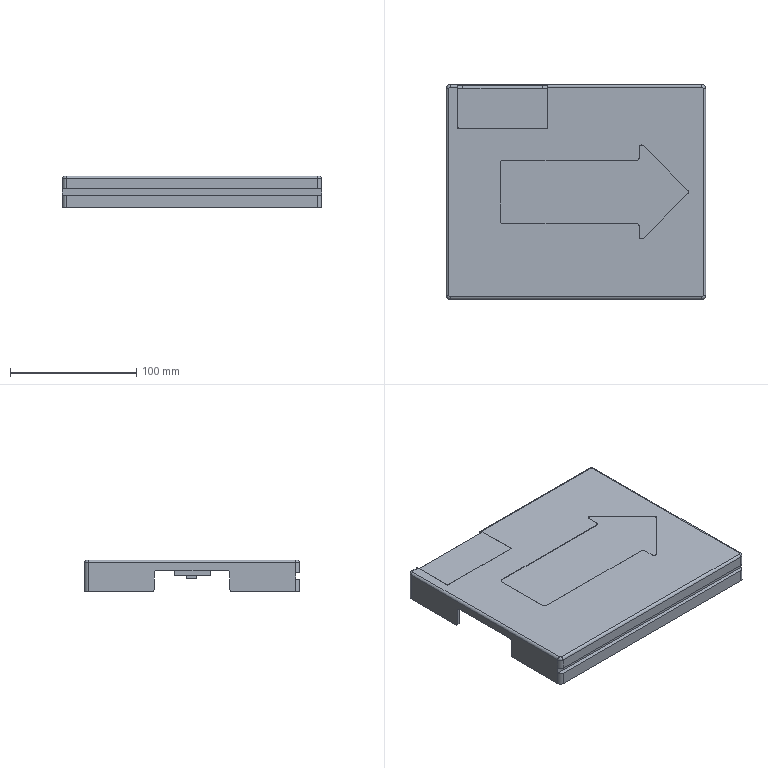NC program | NX | posted with a generic post | part box 205 x 170 x 25 mm
Lines 1976 to 3445 of 3445:
(CAVITY_MILL , TOOL : D4)
N3932 T17 M6
N3934 G54
N3936 G17 G0 G90 X-57.2 Y-18.808 B0. C0. S9500 M3
N3938 G43 Z30. H17
N3940 Z-0.25
N3942 G94 G1 X-57.5 Y-18.981 F1600.
N3944 G3 X-58. Y-19.847 R1.
N3946 G1 Y-23.
N3948 X-54.847
N3950 G3 X-53.981 Y-22.5 R1.
N3952 G1 X-53.808 Y-22.2
N3954 G0 X-57.2 Y-18.808 Z-0.5
N3956 G1 X-57.5 Y-18.981
N3958 G3 X-58. Y-19.847 R1.
N3960 G1 Y-23.
N3962 X-54.847
N3964 G3 X-53.981 Y-22.5 R1.
N3966 G1 X-53.808 Y-22.2
N3968 G0 Z30.
N3970 Y22.2
N3972 Z-0.25
N3974 G1 X-53.981 Y22.5
N3976 G3 X-54.847 Y23. R1.
N3978 G1 X-58.
N3980 Y19.847
N3982 G3 X-57.5 Y18.981 R1.
N3984 G1 X-57.2 Y18.808
N3986 G0 X-53.808 Y22.2 Z-0.5
N3988 G1 X-53.981 Y22.5
N3990 G3 X-54.847 Y23. R1.
N3992 G1 X-58.
N3994 Y19.847
N3996 G3 X-57.5 Y18.981 R1.
N3998 G1 X-57.2 Y18.808
N4000 G0 Z30.
N4002 X-87.339 Y53.756
N4004 Z-0.25
N4006 G1 X-88.048 Y52.529
N4008 G2 X-88.914 Y52.029 R1.
N4010 G1 X-89.48
N4012 Y52.678
N4014 G2 X-91.003 Y54.71 R2.52
N4016 G3 X-91.5 Y55.153 R0.5
N4018 G1 Y52.
N4020 X-88.347
N4022 X-88.348 Y52.029
N4024 X-88.914
N4026 G2 X-89.78 Y52.529 R1.
N4028 G1 X-90.162 Y54.558
N4030 G0 X-87.339 Y53.756 Z-0.5
N4032 G1 X-88.048 Y52.529
N4034 G2 X-88.914 Y52.029 R1.
N4036 G1 X-89.48
N4038 Y52.678
N4040 G2 X-91.003 Y54.71 R2.52
N4042 G3 X-91.5 Y55.153 R0.5
N4044 G1 Y52.
N4046 X-88.347
N4048 X-88.348 Y52.029
N4050 X-88.914
N4052 G2 X-89.78 Y52.529 R1.
N4054 G1 X-90.162 Y54.558
N4056 G0 X-87.339 Y53.756 Z-0.75
N4058 G1 X-88.048 Y52.529
N4060 G2 X-88.914 Y52.029 R1.
N4062 G1 X-89.48
N4064 Y52.678
N4066 G2 X-91.003 Y54.71 R2.52
N4068 G3 X-91.5 Y55.153 R0.5
N4070 G1 Y52.
N4072 X-88.347
N4074 X-88.348 Y52.029
N4076 X-88.914
N4078 G2 X-89.78 Y52.529 R1.
N4080 G1 X-90.162 Y54.558
N4082 G0 X-87.339 Y53.756 Z-1.
N4084 G1 X-88.048 Y52.529
N4086 G2 X-88.914 Y52.029 R1.
N4088 G1 X-89.48
N4090 Y52.678
N4092 G2 X-91.003 Y54.71 R2.52
N4094 G3 X-91.5 Y55.153 R0.5
N4096 G1 Y52.
N4098 X-88.347
N4100 X-88.348 Y52.029
N4102 X-88.914
N4104 G2 X-89.78 Y52.529 R1.
N4106 G1 X-90.162 Y54.558
N4108 G0 Z30.
N4110 X-25.837 Y54.56
N4112 Z-0.25
N4114 G1 X-26.22 Y52.529
N4116 G2 X-27.086 Y52.029 R1.
N4118 G1 X-27.652
N4120 X-27.653 Y52.
N4122 X-24.5
N4124 Y55.153
N4126 G3 X-24.997 Y54.71 R0.5
N4128 G2 X-26.518 Y52.679 R2.52
N4130 G1 X-26.519 Y52.029
N4132 X-27.086
N4134 G2 X-27.952 Y52.529 R1.
N4136 G1 X-28.66 Y53.756
N4138 G0 X-25.837 Y54.56 Z-0.5
N4140 G1 X-26.22 Y52.529
N4142 G2 X-27.086 Y52.029 R1.
N4144 G1 X-27.652
N4146 X-27.653 Y52.
N4148 X-24.5
N4150 Y55.153
N4152 G3 X-24.997 Y54.71 R0.5
N4154 G2 X-26.518 Y52.679 R2.52
N4156 G1 X-26.519 Y52.029
N4158 X-27.086
N4160 G2 X-27.952 Y52.529 R1.
N4162 G1 X-28.66 Y53.756
N4164 G0 X-25.837 Y54.56 Z-0.75
N4166 G1 X-26.22 Y52.529
N4168 G2 X-27.086 Y52.029 R1.
N4170 G1 X-27.652
N4172 X-27.653 Y52.
N4174 X-24.5
N4176 Y55.153
N4178 G3 X-24.997 Y54.71 R0.5
N4180 G2 X-26.518 Y52.679 R2.52
N4182 G1 X-26.519 Y52.029
N4184 X-27.086
N4186 G2 X-27.952 Y52.529 R1.
N4188 G1 X-28.66 Y53.756
N4190 G0 X-25.837 Y54.56 Z-1.
N4192 G1 X-26.22 Y52.529
N4194 G2 X-27.086 Y52.029 R1.
N4196 G1 X-27.652
N4198 X-27.653 Y52.
N4200 X-24.5
N4202 Y55.153
N4204 G3 X-24.997 Y54.71 R0.5
N4206 G2 X-26.518 Y52.679 R2.52
N4208 G1 X-26.519 Y52.029
N4210 X-27.086
N4212 G2 X-27.952 Y52.529 R1.
N4214 G1 X-28.66 Y53.756
N4216 G0 Z30.
N4218 X52.875 Y27.315
N4220 Z-0.25
N4222 G2 X52.497 Y28.218 R1.
N4224 X56.565 Y29.904 R2.52
N4226 G3 X57.23 Y29.942 R0.5
N4228 G1 X52. Y35.172
N4230 Y27.776
N4232 G3 X52.497 Y28.218 R0.5
N4234 G2 X53.093 Y29.021 R1.
N4236 G1 X53.508 Y28.784
N4238 G0 X52.875 Y27.315 Z-0.5
N4240 G2 X52.497 Y28.218 R1.
N4242 X56.565 Y29.904 R2.52
N4244 G3 X57.23 Y29.942 R0.5
N4246 G1 X52. Y35.172
N4248 Y27.776
N4250 G3 X52.497 Y28.218 R0.5
N4252 G2 X53.093 Y29.021 R1.
N4254 G1 X53.508 Y28.784
N4256 G0 Z30.
N4258 X83.642 Y-2.399
N4260 Z-0.25
N4262 G1 X83.976 Y-2.488
N4264 G3 X84.942 Y-2.23 R1.
N4266 G1 X87.172 Y0.
N4268 X84.942 Y2.23
N4270 G3 X83.976 Y2.488 R1.
N4272 G1 X83.642 Y2.399
N4274 G0 Y-2.399 Z-0.5
N4276 G1 X83.976 Y-2.488
N4278 G3 X84.942 Y-2.23 R1.
N4280 G1 X87.172 Y0.
N4282 X84.942 Y2.23
N4284 G3 X83.976 Y2.488 R1.
N4286 G1 X83.642 Y2.399
N4288 G0 Z30.
N4290 X55.021 Y-29.649
N4292 Z-0.25
N4294 G1 X55.027 Y-30.127
N4296 G2 X54.036 Y-30.257 R1.
N4298 X52.497 Y-28.218 R2.52
N4300 G3 X52. Y-27.776 R0.5
N4302 G1 Y-35.172
N4304 X57.23 Y-29.942
N4306 G3 X56.565 Y-29.904 R0.5
N4308 G2 X54.036 Y-30.257 R2.52
N4310 X53.427 Y-29.464 R1.
N4312 G1 X53.769 Y-29.13
N4314 G0 X55.021 Y-29.649 Z-0.5
N4316 G1 X55.027 Y-30.127
N4318 G2 X54.036 Y-30.257 R1.
N4320 X52.497 Y-28.218 R2.52
N4322 G3 X52. Y-27.776 R0.5
N4324 G1 Y-35.135
N4326 X52.002 Y-35.17
N4328 X57.23 Y-29.942
N4330 G3 X56.565 Y-29.904 R0.5
N4332 G2 X54.036 Y-30.257 R2.52
N4334 X53.427 Y-29.464 R1.
N4336 G1 X53.769 Y-29.13
N4338 G0 Z30.
N4340 M5
(FLOOR_WALL_1_COPY_1 , TOOL : D10JING)
N4342 T14 M6
N4344 G54
N4346 G17 G0 G90 X6.616 Y1. B0. C0. S9500 M3
N4348 G43 Z30. H14
N4350 Z1.
N4352 G94 G1 Z-0.5 F1000.
N4354 G3 X5.75 Y1.5 R1.
N4356 G1 X-36.5 F1200.
N4358 Y-1.5
N4360 X48.
N4362 G2 X54.44 Y-2.326 R25.5
N4364 G1 X56.766 Y0.
N4366 X54.44 Y2.326
N4368 G2 X48. Y1.5 R25.5
N4370 G1 X5.75
N4372 Y7.5
N4374 X-42.5
N4376 Y-7.5
N4378 X48.
N4380 G2 X56.024 Y-9.227 R19.5
N4382 G1 X65.251 Y0.
N4384 X56.024 Y9.227
N4386 G2 X48. Y7.5 R19.5
N4388 G1 X5.75
N4390 Y13.5
N4392 X-48.5
N4394 Y-13.5
N4396 X48.
N4398 G2 X56.893 Y-16.843 R13.5
N4400 G1 X73.737 Y0.
N4402 X56.893 Y16.843
N4404 G2 X48. Y13.5 R13.5
N4406 G1 X5.75
N4408 Y19.5
N4410 X-54.5
N4412 Y-19.5
N4414 X48.
N4416 G2 X55.495 Y-26.727 R7.5
N4418 G1 X82.222 Y0.
N4420 X55.495 Y26.727
N4422 G2 X48. Y19.5 R7.5
N4424 G1 X5.75
N4426 X6.616
N4428 G3 X5.75 Y20. R1. F1000.
N4430 G1 X-55. F1200.
N4432 Y-20.
N4434 X48.
N4436 G2 X55. Y-27. R7.
N4438 G1 Y-27.929
N4440 X82.929 Y0.
N4442 X55. Y27.929
N4444 Y27.
N4446 G2 X48. Y20. R7.
N4448 G1 X5.75
N4450 G3 X4.884 Y19.5 R1.
N4452 G1 X4.307 Y18.5
N4454 Z1.
N4456 G0 Z30.
N4458 X-52.029 Y70.
N4460 Z0.6
N4462 G1 X-58. Z-1. F1000.
N4464 X-76. F1200.
N4466 Y67.5
N4468 X-40.
N4470 Y70.
N4472 X-58.
N4474 Y76.
N4476 X-82.
N4478 Y61.5
N4480 X-34.
N4482 Y76.
N4484 X-58.
N4486 Y82.
N4488 X-88.
N4490 Y55.5
N4492 X-28.
N4494 Y82.
N4496 X-58.
N4498 G2 X-58.866 Y82.5 R1.
N4500 G1 X-62.33 Y88.5
N4502 Z0.5
N4504 X-86.5 Y80.5 F8000.
N4506 Z-1. F1000.
N4508 X-88. Y82.866
N4510 G3 X-88.5 Y82. R1.
N4512 G1 Y55. F1200.
N4514 X-27.5
N4516 Y82.
N4518 G3 X-28. Y82.866 R1.
N4520 G1 X-29.5 Y80.5
N4522 Z0.5
N4524 G0 Z30.
(ZLEVEL_PROFILE , TOOL : D10JING)
N4526 X101.868 Y-91.716
N4528 Z-9.5
N4530 G1 Z-12.5 F1000.
N4532 X100.984 Y-90.414
N4534 G3 X100.084 Y-89.979 R1.
N4536 G2 X99.497 Y-90. R8.
N4538 G1 X-99.498
N4540 G2 X-99.784 Y-89.995 R5.003
N4542 X-107.5 Y-81.986 R8.
N4544 G1 Y81.86
N4546 X-107.498
N4548 X-107.5 Y82.
N4550 G2 X-99.498 Y90. R8.
N4552 G1 X99.498
N4554 G2 X107.5 Y82. R8.
N4556 G1 X107.498 Y81.86
N4558 X107.5
N4560 Y-82.
N4562 G2 X100.084 Y-89.979 R8.
N4564 G3 X99.256 Y-90.541 R1.
N4566 G1 X98.55 Y-92.
N4568 Z-9.5
N4570 G0 X101.868 Y-91.716 Z-22.
N4572 G1 Z-25.
N4574 X100.984 Y-90.414
N4576 G3 X100.084 Y-89.979 R1.
N4578 G2 X99.497 Y-90. R8.
N4580 G1 X-99.498
N4582 G2 X-99.784 Y-89.995 R5.003
N4584 X-107.5 Y-81.986 R8.
N4586 G1 Y81.86
N4588 X-107.498
N4590 X-107.5 Y82.
N4592 G2 X-99.498 Y90. R8.
N4594 G1 X99.498
N4596 G2 X107.5 Y82. R8.
N4598 G1 X107.498 Y81.86
N4600 X107.5
N4602 Y-82.
N4604 G2 X100.084 Y-89.979 R8.
N4606 G3 X99.256 Y-90.541 R1.
N4608 G1 X98.55 Y-92.
N4610 Z-22.
N4612 G0 Z30.
N4614 M5
(ZLEVEL_PROFILE_1 , TOOL : D3R0.5)
N4616 T07 M6
N4618 G54
N4620 G17 G0 G90 X-23.737 Y84.233 B0. C0. S9500 M3
N4622 G43 Z30. H7
N4624 Z0.995
N4626 G94 G1 Z-0.005 F1000.
N4628 X-23.304 Y83.999
N4630 G3 X-23.004 Y84.006 R0.3
N4632 G2 X-22.5 Y84.147 R0.952 F2500.
N4634 G1 X99.499
N4636 G2 X101.647 Y82. R2.147
N4638 G1 X101.59 Y-81.871
N4640 X101.647 Y-82.
N4642 G2 X99.499 Y-84.147 R2.147
N4644 G1 X-99.499
N4646 G2 X-101.647 Y-82. R2.147
N4648 G1 X-101.59 Y81.137
N4650 Y81.871
N4652 X-101.647 Y82.
N4654 G2 X-99.499 Y84.147 R2.147
N4656 G1 X-93.5
N4658 G2 X-92.636 Y83.716 R1.144
N4660 G1 X-92.602 Y83.673
N4662 X-92.55 Y83.652
N4664 X-92.496 Y83.661
N4666 X-91.835 Y83.76
N4668 Z0.995
N4670 G0 Z30.
N4672 X-92.331 Y84.413
N4674 Z0.99
N4676 G1 Z-0.01 F1000.
N4678 X-92.701 Y84.13
N4680 G2 X-92.999 Y84.092 R0.3
N4682 G1 X-93.083 Y84.127 F2500.
N4684 X-93.5 Y84.223
N4686 X-99.499
N4688 G3 X-101.723 Y82. R2.223
N4690 G1 X-101.662 Y81.871
N4692 Y81.137
N4694 X-101.723 Y-82.
N4696 G3 X-99.5 Y-84.223 R2.223
N4698 G1 X99.5
N4700 G3 X101.723 Y-82. R2.223
N4702 G1 X101.662 Y-81.871
N4704 X101.723 Y82.
N4706 G3 X99.499 Y84.223 R2.223
N4708 G1 X-22.5
N4710 X-23. Y84.089
N4712 X-23.001 Y84.13 Z-0.013
N4714 Y84.142 Z-0.017
N4716 G2 X-22.5 Y84.287 R0.946
N4718 G1 X99.501
N4720 G2 X101.787 Y82. R2.287
N4722 G1 Y-82.
N4724 G2 X99.501 Y-84.287 R2.287
N4726 G1 X-99.501
N4728 G2 X-101.787 Y-82. R2.287
N4730 G1 Y82.
N4732 G2 X-99.499 Y84.287 R2.287
N4734 G1 X-93.5
N4736 X-93.073 Y84.197
N4738 X-92.996 Y84.143
N4740 X-92.987 Y84.197 Z-0.024
N4742 X-93.066 Y84.248
N4744 X-93.5 Y84.346
N4746 X-99.499
N4748 G3 X-101.846 Y82. R2.346
N4750 G1 Y-82.
N4752 G3 X-99.499 Y-84.346 R2.346
N4754 G1 X99.499
N4756 G3 X101.846 Y-82. R2.346
N4758 G1 Y82.
N4760 G3 X99.499 Y84.346 R2.346
N4762 G1 X-22.5
N4764 G3 X-23.001 Y84.202 R0.892
N4766 G1 Y84.277 Z-0.033
N4768 X-22.925 Y84.318
N4770 X-22.5 Y84.407
N4772 X99.499
N4774 G2 X101.907 Y82. R2.407
N4776 G1 Y-82.
N4778 G2 X99.499 Y-84.407 R2.407
N4780 G1 X-99.499
N4782 G2 X-101.907 Y-82. R2.407
N4784 G1 Y82.
N4786 G2 X-99.499 Y84.407 R2.407
N4788 G1 X-93.5
N4790 X-93.058 Y84.312
N4792 X-92.975 Y84.264
N4794 X-93. Y84.348 Z-0.045
N4796 G3 X-93.5 Y84.474 R2.086
N4798 G1 X-99.499
N4800 G3 X-101.974 Y82. R2.474
N4802 G1 Y-82.
N4804 G3 X-99.5 Y-84.474 R2.474
N4806 G1 X99.5
N4808 G3 X101.974 Y-82. R2.474
N4810 G1 Y82.
N4812 G3 X99.499 Y84.474 R2.474
N4814 G1 X-22.5
N4816 G3 X-23.001 Y84.35 R1.112
N4818 G1 Y84.421 Z-0.061
N4820 G2 X-22.5 Y84.549 R1.049
N4822 G1 X99.499
N4824 G2 X102.049 Y82. R2.549
N4826 G1 Y-82.
N4828 G2 X99.501 Y-84.549 R2.549
N4830 G1 X-99.501
N4832 G2 X-102.049 Y-82. R2.549
N4834 G1 Y82.
N4836 G2 X-99.501 Y84.549 R2.549
N4838 G1 X-93.5
N4840 G2 X-93. Y84.419 R2.188
N4842 G1 Y84.507 Z-0.081
N4844 G3 X-93.5 Y84.63 R1.14
N4846 G1 X-99.5
N4848 G3 X-102.13 Y82. R2.63
N4850 G1 Y-82.
N4852 G3 X-99.499 Y-84.63 R2.63
N4854 G1 X99.499
N4856 G3 X102.13 Y-82. R2.63
N4858 G1 Y82.
N4860 G3 X99.5 Y84.63 R2.63
N4862 G1 X-22.5
N4864 G3 X-23.001 Y84.509 R1.123
N4866 G1 X-22.963 Y84.572 Z-0.092
N4868 X-22.916 Y84.61 Z-0.104
N4870 X-22.5 Y84.697
N4872 X99.5
N4874 G2 X102.197 Y82. R2.697
N4876 G1 Y-82.
N4878 G2 X99.5 Y-84.697 R2.697
N4880 G1 X-99.5
N4882 G2 X-102.197 Y-82. R2.697
N4884 G1 Y82.
N4886 G2 X-99.5 Y84.697 R2.697
N4888 G1 X-93.5
N4890 X-93. Y84.579
N4892 Y84.639 Z-0.117
N4894 Y84.673 Z-0.13
N4896 X-93.5 Y84.795
N4898 X-99.5
N4900 G3 X-102.295 Y82. R2.795
N4902 G1 Y-82.
N4904 G3 X-99.501 Y-84.795 R2.795
N4906 G1 X99.501
N4908 G3 X102.295 Y-82. R2.795
N4910 G1 Y82.
N4912 G3 X99.5 Y84.795 R2.795
N4914 G1 X-22.5
N4916 X-22.921 Y84.704
N4918 X-22.948 Y84.782 Z-0.158
N4920 X-22.868 Y84.816
N4922 X-22.5 Y84.875
N4924 X99.5
N4926 G2 X102.375 Y82. R2.875
N4928 G1 Y-82.
N4930 G2 X99.499 Y-84.875 R2.875
N4932 G1 X-99.499
N4934 G2 X-102.375 Y-82. R2.875
N4936 G1 Y82.
N4938 G2 X-99.5 Y84.875 R2.875
N4940 G1 X-93.5
N4942 X-93.058 Y84.786
N4944 X-93. Y84.76
N4946 X-92.999 Y84.853 Z-0.192
N4948 X-93.5 Y84.96
N4950 X-99.5
N4952 G3 X-102.46 Y82. R2.96
N4954 G1 Y-82.
N4956 G3 X-99.5 Y-84.96 R2.96
N4958 G1 X99.5
N4960 G3 X102.46 Y-82. R2.96
N4962 G1 Y82.
N4964 G3 X99.5 Y84.96 R2.96
N4966 G1 X-22.5
N4968 G3 X-23. Y84.846 R8.99
N4970 G1 Y84.898 Z-0.21
N4972 X-23.001 Y84.931 Z-0.229
N4974 G2 X-22.5 Y85.045 R1.121
N4976 G1 X99.5
N4978 G2 X102.545 Y82. R3.045
N4980 G1 Y-82.
N4982 G2 X99.501 Y-85.045 R3.045
N4984 G1 X-99.501
N4986 G2 X-102.545 Y-82. R3.045
N4988 G1 Y82.
N4990 G2 X-99.5 Y85.045 R3.045
N4992 G1 X-93.5
N4994 X-92.999 Y84.943
N4996 Y84.984 Z-0.249
N4998 X-93. Y85.025 Z-0.269
N5000 X-93.084 Y85.053
N5002 X-93.5 Y85.129
N5004 X-99.5
N5006 G3 X-102.629 Y82. R3.129
N5008 G1 Y-82.
N5010 G3 X-99.5 Y-85.129 R3.129
N5012 G1 X99.5
N5014 G3 X102.629 Y-82. R3.129
N5016 G1 Y82.
N5018 G3 X99.5 Y85.129 R3.129
N5020 G1 X-22.5
N5022 X-22.923 Y85.053
N5024 X-23.001 Y85.022
N5026 X-22.943 Y85.083 Z-0.291
N5028 X-22.885 Y85.142 Z-0.313
N5030 X-22.5 Y85.212
N5032 X99.5
N5034 G2 X102.712 Y82. R3.212
N5036 G1 Y-82.
N5038 G2 X99.5 Y-85.212 R3.212
N5040 G1 X-99.5
N5042 G2 X-102.712 Y-82. R3.212
N5044 G1 Y82.
N5046 G2 X-99.5 Y85.212 R3.212
N5048 G1 X-93.5
N5050 G2 X-93. Y85.109 R5.057
N5052 G1 Y85.152 Z-0.337
N5054 Y85.197 Z-0.361
N5056 G3 X-93.5 Y85.294 R5.188
N5058 G1 X-99.5
N5060 G3 X-102.794 Y82. R3.294
N5062 G1 Y-82.
N5064 G3 X-99.501 Y-85.294 R3.294
N5066 G1 X99.501
N5068 G3 X102.794 Y-82. R3.294
N5070 G1 Y82.
N5072 G3 X99.5 Y85.294 R3.294
N5074 G1 X-22.5
N5076 X-22.885 Y85.23
N5078 X-22.939 Y85.256 Z-0.387
N5080 X-22.995 Y85.295 Z-0.412
N5082 X-22.5 Y85.375
N5084 X99.5
N5086 G2 X102.875 Y82. R3.375
N5088 G1 Y-82.
N5090 G2 X99.5 Y-85.375 R3.375
N5092 G1 X-99.5
N5094 G2 X-102.875 Y-82. R3.375
N5096 G1 Y82.
N5098 G2 X-99.5 Y85.375 R3.375
N5100 G1 X-93.5
N5102 X-93. Y85.292
N5104 Y85.342 Z-0.44
N5106 X-92.999 Y85.376 Z-0.467
N5108 X-93.5 Y85.455
N5110 X-99.5
N5112 G3 X-102.955 Y82. R3.455
N5114 G1 Y-82.
N5116 G3 X-99.5 Y-85.455 R3.455
N5118 G1 X99.5
N5120 G3 X102.955 Y-82. R3.455
N5122 G1 Y82.
N5124 G3 X99.5 Y85.455 R3.455
N5126 G1 X-22.5
N5128 X-23.002 Y85.378
N5130 Y85.419 Z-0.496
N5132 Y85.457 Z-0.525
N5134 X-22.5 Y85.533
N5136 X99.5
N5138 G2 X103.033 Y82. R3.533
N5140 G1 Y-82.
N5142 G2 X99.501 Y-85.533 R3.533
N5144 G1 X-99.501
N5146 G2 X-103.033 Y-82. R3.533
N5148 G1 Y82.
N5150 G2 X-99.5 Y85.533 R3.533
N5152 G1 X-93.5
N5154 X-92.999 Y85.455
N5156 X-93. Y85.494 Z-0.556
N5158 Y85.53 Z-0.586
N5160 X-93.058 Y85.542
N5162 X-93.5 Y85.609
N5164 X-99.5
N5166 G3 X-103.109 Y82. R3.609
N5168 G1 Y-82.
N5170 G3 X-99.5 Y-85.609 R3.609
N5172 G1 X99.5
N5174 G3 X103.109 Y-82. R3.609
N5176 G1 Y82.
N5178 G3 X99.5 Y85.609 R3.609
N5180 G1 X-22.5
N5182 G3 X-23. Y85.532 R22.548
N5184 G1 Y85.57 Z-0.618
N5186 Y85.605 Z-0.651
N5188 X-22.5 Y85.682
N5190 X99.5
N5192 G2 X103.182 Y82. R3.682
N5194 G1 Y-82.
N5196 G2 X99.5 Y-85.682 R3.682
N5198 G1 X-99.5
N5200 G2 X-103.182 Y-82. R3.682
N5202 G1 Y82.
N5204 G2 X-99.5 Y85.682 R3.682
N5206 G1 X-93.5
N5208 X-93. Y85.603
N5210 Y85.65 Z-0.684
N5212 Y85.679 Z-0.718
N5214 X-93.5 Y85.753
N5216 X-99.5
N5218 G3 X-103.253 Y82. R3.753
N5220 G1 Y-82.
N5222 G3 X-99.501 Y-85.753 R3.753
N5224 G1 X99.501
N5226 G3 X103.253 Y-82. R3.753
N5228 G1 Y82.
N5230 G3 X99.5 Y85.753 R3.753
N5232 G1 X-22.5
N5234 X-23. Y85.68
N5236 Y85.726 Z-0.753
N5238 Y85.759 Z-0.788
N5240 X-22.5 Y85.822
N5242 X99.5
N5244 G2 X103.322 Y82. R3.822
N5246 G1 Y-82.
N5248 G2 X99.5 Y-85.822 R3.822
N5250 G1 X-99.5
N5252 G2 X-103.322 Y-82. R3.822
N5254 G1 Y82.
N5256 G2 X-99.5 Y85.822 R3.822
N5258 G1 X-93.5
N5260 X-93. Y85.757
N5262 Y85.794 Z-0.825
N5264 Y85.825 Z-0.862
N5266 X-93.5 Y85.888
N5268 X-99.5
N5270 G3 X-103.388 Y82. R3.888
N5272 G1 Y-82.
N5274 G3 X-99.5 Y-85.888 R3.888
N5276 G1 X99.5
N5278 G3 X103.388 Y-82. R3.888
N5280 G1 Y82.
N5282 G3 X99.5 Y85.888 R3.888
N5284 G1 X-22.5
N5286 X-23. Y85.827
N5288 Y85.857 Z-0.9
N5290 Y85.889 Z-0.938
N5292 X-22.5 Y85.952
N5294 X99.5
N5296 G2 X103.452 Y82. R3.952
N5298 G1 Y-82.
N5300 G2 X99.501 Y-85.952 R3.952
N5302 G1 X-99.501
N5304 G2 X-103.452 Y-82. R3.952
N5306 G1 Y82.
N5308 G2 X-99.5 Y85.952 R3.952
N5310 G1 X-93.5
N5312 G2 X-93. Y85.887 R5.712
N5314 G1 Y85.92 Z-0.977
N5316 Y85.952 Z-1.016
N5318 X-93.5 Y86.012
N5320 X-99.5
N5322 G3 X-103.512 Y82. R4.012
N5324 G1 Y-82.
N5326 G3 X-99.501 Y-86.012 R4.012
N5328 G1 X99.501
N5330 G3 X103.512 Y-82. R4.012
N5332 G1 Y82.
N5334 G3 X99.5 Y86.012 R4.012
N5336 G1 X-22.5
N5338 X-23. Y85.953
N5340 Y85.986 Z-1.057
N5342 Y86.019 Z-1.098
N5344 X-22.5 Y86.07
N5346 X99.5
N5348 G2 X103.57 Y82. R4.07
N5350 G1 Y-82.
N5352 G2 X99.5 Y-86.07 R4.07
N5354 G1 X-99.5
N5356 G2 X-103.57 Y-82. R4.07
N5358 G1 Y82.
N5360 G2 X-99.5 Y86.07 R4.07
N5362 G1 X-93.5
N5364 X-93. Y86.018
N5366 Y86.044 Z-1.139
N5368 Y86.068 Z-1.181
N5370 X-93.5 Y86.124
N5372 X-99.5
N5374 G3 X-103.624 Y82. R4.124
N5376 G1 Y-82.
N5378 G3 X-99.5 Y-86.124 R4.124
N5380 G1 X99.5
N5382 G3 X103.624 Y-82. R4.124
N5384 G1 Y82.
N5386 G3 X99.5 Y86.124 R4.124
N5388 G1 X-22.5
N5390 X-22.762 Y86.096
N5392 X-22.892 Y86.07
N5394 X-22.918 Y86.057
N5396 X-22.944 Y86.069
N5398 X-22.945 Y86.097 Z-1.224
N5400 Y86.115 Z-1.267
N5402 X-22.883 Y86.117
N5404 X-22.822 Y86.136
N5406 X-22.762 Y86.15
N5408 X-22.5 Y86.175
N5410 X99.5
N5412 G2 X103.675 Y82. R4.175
N5414 G1 Y-82.
N5416 G2 X99.5 Y-86.175 R4.175
N5418 G1 X-99.5
N5420 G2 X-103.675 Y-82. R4.175
N5422 G1 Y82.
N5424 G2 X-99.5 Y86.175 R4.175
N5426 G1 X-93.5
N5428 G2 X-93. Y86.114 R6.38
N5430 G1 Y86.143 Z-1.31
N5432 Y86.161 Z-1.354
N5434 G3 X-93.5 Y86.222 R5.652
N5436 G1 X-99.5
N5438 G3 X-103.722 Y82. R4.222
N5440 G1 X-103.715 Y81.871
N5442 Y-81.871
N5444 X-103.722 Y-82.
N5446 G3 X-99.501 Y-86.222 R4.222
N5448 G1 X99.501
N5450 G3 X103.722 Y-82. R4.222
N5452 G1 X103.715 Y-81.871
N5454 Y81.871
N5456 X103.722 Y82.
N5458 G3 X99.5 Y86.222 R4.222
N5460 G1 X-22.5
N5462 X-22.762 Y86.194
N5464 X-22.823 Y86.183
N5466 X-22.884 Y86.164
N5468 X-22.946 Y86.163
N5470 Y86.191 Z-1.398
N5472 Y86.211 Z-1.443
N5474 X-22.905 Y86.213
N5476 X-22.762 Y86.238
N5478 X-22.5 Y86.266
N5480 X99.5
N5482 G2 X103.766 Y82. R4.266
N5484 G1 Y-82.
N5486 G2 X99.501 Y-86.266 R4.266
N5488 G1 X-99.501
N5490 G2 X-103.766 Y-82. R4.266
N5492 G1 Y82.
N5494 G2 X-99.5 Y86.266 R4.266
N5496 G1 X-93.5
N5498 X-93. Y86.209
N5500 Y86.237 Z-1.488
N5502 Y86.257 Z-1.533
N5504 X-93.5 Y86.306
N5506 X-99.5
N5508 G3 X-103.806 Y82. R4.306
N5510 G1 X-103.8 Y81.871
N5512 Y-81.871
N5514 X-103.806 Y-82.
N5516 G3 X-99.5 Y-86.306 R4.306
N5518 G1 X99.5
N5520 G3 X103.806 Y-82. R4.306
N5522 G1 X103.8 Y-81.871
N5524 Y81.871
N5526 X103.806 Y82.
N5528 G3 X99.5 Y86.306 R4.306
N5530 G1 X-22.5
N5532 G2 X-22.947 Y86.26 R21.539
N5534 G1 X-22.998 Y86.296 Z-1.626
N5536 G3 X-22.5 Y86.342 R8.812
N5538 G1 X99.5
N5540 G2 X103.842 Y82. R4.342
N5542 G1 X103.836 Y81.871
N5544 Y-81.871
N5546 X103.842 Y-82.
N5548 G2 X99.5 Y-86.342 R4.342
N5550 G1 X-99.5
N5552 G2 X-103.842 Y-82. R4.342
N5554 G1 X-103.836 Y-81.871
N5556 Y81.871
N5558 X-103.842 Y82.
N5560 G2 X-99.5 Y86.342 R4.342
N5562 G1 X-93.5
N5564 X-93. Y86.297
N5566 X-92.999 Y86.314 Z-1.673
N5568 Y86.33 Z-1.72
N5570 X-93.5 Y86.375
N5572 X-99.5
N5574 G3 X-103.875 Y82. R4.375
N5576 G1 Y-82.
N5578 G3 X-99.5 Y-86.375 R4.375
N5580 G1 X99.5
N5582 G3 X103.875 Y-82. R4.375
N5584 G1 Y82.
N5586 G3 X99.5 Y86.375 R4.375
N5588 G1 X-22.5
N5590 G2 X-22.998 Y86.326 R10.836
N5592 G1 Y86.342 Z-1.768
N5594 X-22.999 Y86.357 Z-1.816
N5596 G3 X-22.5 Y86.405 R15.059
N5598 G1 X99.5
N5600 G2 X103.905 Y82. R4.405
N5602 G1 Y-82.
N5604 G2 X99.5 Y-86.405 R4.405
N5606 G1 X-99.5
N5608 G2 X-103.905 Y-82. R4.405
N5610 G1 Y82.
N5612 G2 X-99.5 Y86.405 R4.405
N5614 G1 X-93.5
N5616 X-92.997 Y86.363
N5618 Y86.381 Z-1.864
N5620 Y86.395 Z-1.913
N5622 X-93.5 Y86.43
N5624 X-99.5
N5626 G3 X-103.93 Y82. R4.43
N5628 G1 Y-82.
N5630 G3 X-99.501 Y-86.43 R4.43
N5632 G1 X99.501
N5634 G3 X103.93 Y-82. R4.43
N5636 G1 Y82.
N5638 G3 X99.5 Y86.43 R4.43
N5640 G1 X-22.5
N5642 G2 X-22.999 Y86.388 R9.05
N5644 G1 X-23. Y86.405 Z-1.961
N5646 Y86.414 Z-2.01
N5648 X-22.5 Y86.452
N5650 X99.5
N5652 G2 X103.952 Y82. R4.452
N5654 G1 Y-82.
N5656 G2 X99.501 Y-86.452 R4.452
N5658 G1 X-99.501
N5660 G2 X-103.952 Y-82. R4.452
N5662 G1 Y82.
N5664 G2 X-99.5 Y86.452 R4.452
N5666 G1 X-93.5
N5668 X-92.997 Y86.422
N5670 Y86.433 Z-2.059
N5672 X-92.996 Y86.446 Z-2.109
N5674 G2 X-93.5 Y86.469 R5.396
N5676 G1 X-99.5
N5678 G3 X-103.969 Y82. R4.469
N5680 G1 Y-82.
N5682 G3 X-99.501 Y-86.469 R4.469
N5684 G1 X99.501
N5686 G3 X103.969 Y-82. R4.469
N5688 G1 Y82.
N5690 G3 X99.5 Y86.469 R4.469
N5692 G1 X-22.5
N5694 X-23. Y86.44
N5696 X-23.001 Y86.451 Z-2.158
N5698 Y86.459 Z-2.206
N5700 X-22.518 Y86.479
N5702 X-22.5 Y86.483
N5704 X99.5
N5706 G2 X103.983 Y82. R4.483
N5708 G1 X103.977 Y81.871
N5710 Y-81.871
N5712 X103.983 Y-82.
N5714 G2 X99.501 Y-86.483 R4.483
N5716 G1 X-99.501
N5718 G2 X-103.983 Y-82. R4.483
N5720 G1 X-103.977 Y-81.871
N5722 Y81.871
N5724 X-103.983 Y82.
N5726 G2 X-99.5 Y86.483 R4.483
N5728 G1 X-93.5
N5730 G3 X-92.996 Y86.465 R6.436
N5732 G1 X-92.997 Y86.472 Z-2.255
N5734 Y86.476 Z-2.304
N5736 G2 X-93.5 Y86.492 R3.383
N5738 G1 X-99.5
N5740 G3 X-103.992 Y82. R4.492
N5742 G1 X-103.986 Y81.871
N5744 Y-81.871
N5746 X-103.992 Y-82.
N5748 G3 X-99.501 Y-86.492 R4.492
N5750 G1 X99.501
N5752 G3 X103.992 Y-82. R4.492
N5754 G1 X103.986 Y-81.871
N5756 Y81.871
N5758 X103.992 Y82.
N5760 G3 X99.5 Y86.492 R4.492
N5762 G1 X-22.5
N5764 G2 X-23.001 Y86.473 R5.056
N5766 G1 Y86.481 Z-2.402
N5768 G3 X-22.5 Y86.498 R4.446
N5770 G1 X99.5
N5772 G2 X103.998 Y82. R4.498
N5774 G1 Y-82.
N5776 G2 X100.84 Y-86.294 R4.498
N5778 X99.512 Y-86.496 R4.458
N5780 G1 X-99.527
N5782 G2 X-100.108 Y-86.457 R4.301
N5784 X-103.882 Y-83.016 R4.498
N5786 X-103.995 Y-82.024 R4.393
N5788 G1 Y82.023
N5790 G2 X-103.872 Y83.057 R4.401
N5792 X-99.5 Y86.498 R4.498
N5794 G1 X-93.5
N5796 G3 X-92.999 Y86.483 R3.22
N5798 G1 X-93. Y86.487 Z-2.5
N5800 G2 X-93.5 Y86.498 R5.814
N5802 G1 X-93.742 Y86.5
N5804 X-99.494 Y86.498
N5806 G3 X-102.472 Y85.385 R4.54
N5808 G1 X-102.803 Y85.053
N5810 X-103.014 Y84.808
N5812 G3 X-103.354 Y84.319 R4.234
N5814 X-103.816 Y83.264 R4.645
N5816 X-103.996 Y82.016 R4.415
N5818 G1 Y-82.008
N5820 G3 X-103.801 Y-83.315 R4.48
N5822 G1 X-103.772 Y-83.407
N5824 G3 X-103.636 Y-83.77 R4.071
N5826 X-101.996 Y-85.742 R4.519
N5828 G1 X-101.778 Y-85.881
N5830 G3 X-100.835 Y-86.295 R4.716
N5832 X-99.526 Y-86.496 R4.365
N5834 G1 X99.544
N5836 G3 X100.839 Y-86.295 R4.258
N5838 X101.421 Y-86.067 R4.932
N5840 G1 X101.784 Y-85.88
N5842 X102.116 Y-85.661
N5844 X102.274 Y-85.542
N5846 X102.56 Y-85.298
N5848 X102.596 Y-85.262
N5850 G3 X103.997 Y-82.014 R4.465
N5852 G1 Y82.011
N5854 G3 X99.509 Y86.498 R4.487
N5856 G1 X-22.273 Y86.499
N5858 G3 X-23.001 Y86.485 R212.703
N5860 G2 X-23.264 Y86.629 R0.3
N5862 G1 X-23.505 Y87.025
N5864 Z-1.5
N5866 G0 Z30.
(ZLEVEL_PROFILE_1_COPY , TOOL : D3R0.5)
N5868 X-91.261 Y83.817
N5870 Z-0.009
N5872 G1 Z-1.009 F1000.
N5874 X-91.85 Y83.476
N5876 G3 X-92. Y83.217 R0.3
N5878 G1 X-89.499 F2500.
N5880 X-26.501
N5882 X-24.
N5884 Y83.261 Z-1.014
N5886 Y83.299 Z-1.018
N5888 Y83.333 Z-1.022
N5890 X-26.501
N5892 X-89.499
N5894 X-92.
N5896 Y83.439 Z-1.039
N5898 X-89.499
N5900 X-26.501
N5902 X-24.
N5904 Y83.476 Z-1.046
N5906 Y83.51 Z-1.053
N5908 Y83.542 Z-1.059
N5910 X-26.501
N5912 X-89.499
N5914 X-92.
N5916 Y83.637 Z-1.084
N5918 X-89.499
N5920 X-26.501
N5922 X-24.
N5924 Y83.741 Z-1.112
N5926 X-26.501
N5928 X-89.499
N5930 X-92.
N5932 Y83.837 Z-1.144
N5934 X-89.499
N5936 X-26.501
N5938 X-24.
N5940 Y83.932 Z-1.18
N5942 X-26.501
N5944 X-89.499
N5946 X-92.
N5948 Y84.025 Z-1.22
N5950 X-89.499
N5952 X-26.501
N5954 X-24.
N5956 Y84.117 Z-1.263
N5958 X-26.501
N5960 X-89.499
N5962 X-92.
N5964 Y84.206 Z-1.31
N5966 X-89.499
N5968 X-26.501
N5970 X-24.
N5972 Y84.293 Z-1.36
N5974 X-26.501
N5976 X-89.499
N5978 X-92.
N5980 Y84.378 Z-1.414
N5982 X-89.499
N5984 X-26.501
N5986 X-24.
N5988 Y84.461 Z-1.471
N5990 X-26.501
N5992 X-89.499
N5994 X-92.
N5996 Y84.541 Z-1.532
N5998 X-89.499
N6000 X-26.501
N6002 X-24.
N6004 Y84.619 Z-1.595
N6006 X-26.501
N6008 X-89.499
N6010 X-92.
N6012 Y84.694 Z-1.661
N6014 X-89.499
N6016 X-26.501
N6018 X-24.
N6020 Y84.766 Z-1.731
N6022 X-26.501
N6024 X-89.499
N6026 X-92.
N6028 X-91.998 Y84.836 Z-1.803
N6030 X-89.499
N6032 X-26.501
N6034 X-24.002
N6036 X-24.001 Y84.902 Z-1.878
N6038 X-26.501
N6040 X-89.499
N6042 X-91.999
N6044 Y84.966 Z-1.956
N6046 X-89.499
N6048 X-26.501
N6050 X-24.001
N6052 X-23.999 Y85.026 Z-2.036
N6054 X-26.501
N6056 X-89.499
N6058 X-92.001
N6060 X-92.004 Y85.083 Z-2.118
N6062 X-89.499
N6064 X-26.501
N6066 X-23.996
N6068 X-23.992 Y85.137 Z-2.203
N6070 X-26.501
N6072 X-89.499
N6074 X-92.008
N6076 X-92.013 Y85.187 Z-2.289
N6078 X-89.499
N6080 X-26.501
N6082 X-23.988
N6084 X-23.982 Y85.234 Z-2.378
N6086 X-26.501
N6088 X-89.499
N6090 X-92.019
N6092 X-92.057 Y85.406
N6094 Y85.409 Z-2.468
N6096 X-92.047 Y85.372
N6098 X-92.045
N6100 X-92.026 Y85.277
N6102 X-89.499
N6104 X-26.501
N6106 X-23.974
N6108 X-23.966 Y85.317 Z-2.56
N6110 X-26.501
N6112 X-89.499
N6114 X-92.034
N6116 X-92.047 Y85.372
N6118 X-92.05 Y85.384 Z-2.653
N6120 X-92.031 Y85.352
N6122 X-89.499
N6124 X-26.501
N6126 X-23.958
N6128 X-23.95 Y85.384 Z-2.748
N6130 X-26.501
N6132 X-89.499
N6134 X-92.05
N6136 X-92.058 Y85.412 Z-2.844
N6138 X-89.499
N6140 X-26.501
N6142 X-23.942
N6144 X-23.935 Y85.437 Z-2.941
N6146 X-26.501
N6148 X-89.499
N6150 X-92.065
N6152 X-92.071 Y85.457 Z-3.039
N6154 X-89.499
N6156 X-26.501
N6158 X-23.929
N6160 X-23.923 Y85.474 Z-3.138
N6162 X-26.501
N6164 X-89.499
N6166 X-92.077
N6168 X-92.081 Y85.485 Z-3.228
N6170 X-89.499
N6172 X-26.501
N6174 X-23.919
N6176 X-23.917 Y85.493 Z-3.319
N6178 X-26.501
N6180 X-89.499
N6182 X-92.083
N6184 X-92.085 Y85.498 Z-3.409
N6186 X-89.499
N6188 X-26.501
N6190 X-23.915
N6192 X-23.905 Y85.526 Z-3.5
N6194 X-23.929 Y85.5
N6196 X-92.071
N6198 X-92.095 Y85.526
N6200 Z-2.5
N6202 G0 Z30.
N6204 M5
(PLANAR_MILL_COPY_COPY , TOOL : D6A45)
N6206 T01 M6
N6208 G54
N6210 G17 G0 G90 X-92.3 Y85.866 B0. C0. S9500 M3
N6212 G43 Z30. H1
N6214 Z0.2
N6216 G94 G1 Z-0.8 F1250.
N6218 G3 X-92.8 Y85. R1.
N6220 G1 Y52.
N6222 G3 X-91.5 Y50.7 R1.3
N6224 G1 X-24.5
N6226 G3 X-23.2 Y52. R1.3
N6228 G1 Y85.
N6230 G3 X-23.7 Y85.866 R1.
N6232 G1 Z0.2
N6234 G0 Z30.
(PLANAR_MILL_COPY_COPY_COPY , TOOL : D6A45)
N6236 X-4.134 Y24.2
N6238 Z0.65
N6240 G1 Z-0.35
N6242 G3 X-5. Y24.7 R1.
N6244 G1 X-58.
N6246 G3 X-59.7 Y23. R1.7
N6248 G1 Y-23.
N6250 G3 X-58. Y-24.7 R1.7
N6252 G1 X48.
N6254 G2 X50.3 Y-27. R2.3
N6256 G1 Y-35.172
N6258 G3 X53.202 Y-36.374 R1.7
N6260 G1 X88.374 Y-1.202
N6262 G3 X88.374 Y1.202 R1.7
N6264 G1 X53.202 Y36.374
N6266 G3 X50.3 Y35.172 R1.7
N6268 G1 Y27.
N6270 G2 X48. Y24.7 R2.3
N6272 G1 X-5.
N6274 G3 X-5.866 Y24.2 R1.
N6276 G1 Z0.65
N6278 G0 Z30.
N6280 M5
(PLANAR_MILL_1 , TOOL : T10H1.5)
N6282 T13 M6
N6284 G54
N6286 G17 G0 G90 X105.964 Y-95. B0. C0. S6500 M3
N6288 G43 Z30. H13
N6290 Z-11.5
N6292 G94 G1 X103.366 Y-90.5 F1250.
N6294 G3 X102.5 Y-90. R1.
N6296 G1 X-102.5
N6298 G3 X-103.366 Y-90.5 R1.
N6300 G1 X-105.964 Y-95.
N6302 G0 X106.137
N6304 G1 X103.366 Y-90.2
N6306 G3 X102.5 Y-89.7 R1.
N6308 G1 X-102.5
N6310 G3 X-103.366 Y-90.2 R1.
N6312 G1 X-106.137 Y-95.
N6314 G0 X106.311
N6316 G1 X103.366 Y-89.9
N6318 G3 X102.5 Y-89.4 R1.
N6320 G1 X-102.5
N6322 G3 X-103.366 Y-89.9 R1.
N6324 G1 X-106.311 Y-95.
N6326 G0 X106.484
N6328 G1 X103.366 Y-89.6
N6330 G3 X102.5 Y-89.1 R1.
N6332 G1 X-102.5
N6334 G3 X-103.366 Y-89.6 R1.
N6336 G1 X-106.484 Y-95.
N6338 G0 X106.657
N6340 G1 X103.366 Y-89.3
N6342 G3 X102.5 Y-88.8 R1.
N6344 G1 X-102.5
N6346 G3 X-103.366 Y-89.3 R1.
N6348 G1 X-106.657 Y-95.
N6350 G0 X106.83
N6352 G1 X103.366 Y-89.
N6354 G3 X102.5 Y-88.5 R1.
N6356 G1 X-102.5
N6358 G3 X-103.366 Y-89. R1.
N6360 G1 X-106.83 Y-95.
N6362 G0 X107.003
N6364 G1 X103.366 Y-88.7
N6366 G3 X102.5 Y-88.2 R1.
N6368 G1 X-102.5
N6370 G3 X-103.366 Y-88.7 R1.
N6372 G1 X-107.003 Y-95.
N6374 G0 X107.177
N6376 G1 X103.366 Y-88.4
N6378 G3 X102.5 Y-87.9 R1.
N6380 G1 X-102.5
N6382 G3 X-103.366 Y-88.4 R1.
N6384 G1 X-107.177 Y-95.
N6386 G0 X107.35
N6388 G1 X103.366 Y-88.1
N6390 G3 X102.5 Y-87.6 R1.
N6392 G1 X-102.5
N6394 G3 X-103.366 Y-88.1 R1.
N6396 G1 X-107.35 Y-95.
N6398 G0 X107.523
N6400 G1 X103.366 Y-87.8
N6402 G3 X102.5 Y-87.3 R1.
N6404 G1 X-102.5
N6406 G3 X-103.366 Y-87.8 R1.
N6408 G1 X-107.523 Y-95.
N6410 G0 X107.696
N6412 G1 X103.366 Y-87.5
N6414 G3 X102.5 Y-87. R1.
N6416 G1 X-102.5
N6418 G3 X-103.366 Y-87.5 R1.
N6420 G1 X-107.696 Y-95.
N6422 G0 X105.964 Z-12.667
N6424 G1 X103.366 Y-90.5
N6426 G3 X102.5 Y-90. R1.
N6428 G1 X-102.5
N6430 G3 X-103.366 Y-90.5 R1.
N6432 G1 X-105.964 Y-95.
N6434 G0 X106.137
N6436 G1 X103.366 Y-90.2
N6438 G3 X102.5 Y-89.7 R1.
N6440 G1 X-102.5
N6442 G3 X-103.366 Y-90.2 R1.
N6444 G1 X-106.137 Y-95.
N6446 G0 X106.311
N6448 G1 X103.366 Y-89.9
N6450 G3 X102.5 Y-89.4 R1.
N6452 G1 X-102.5
N6454 G3 X-103.366 Y-89.9 R1.
N6456 G1 X-106.311 Y-95.
N6458 G0 X106.484
N6460 G1 X103.366 Y-89.6
N6462 G3 X102.5 Y-89.1 R1.
N6464 G1 X-102.5
N6466 G3 X-103.366 Y-89.6 R1.
N6468 G1 X-106.484 Y-95.
N6470 G0 X106.657
N6472 G1 X103.366 Y-89.3
N6474 G3 X102.5 Y-88.8 R1.
N6476 G1 X-102.5
N6478 G3 X-103.366 Y-89.3 R1.
N6480 G1 X-106.657 Y-95.
N6482 G0 X106.83
N6484 G1 X103.366 Y-89.
N6486 G3 X102.5 Y-88.5 R1.
N6488 G1 X-102.5
N6490 G3 X-103.366 Y-89. R1.
N6492 G1 X-106.83 Y-95.
N6494 G0 X107.003
N6496 G1 X103.366 Y-88.7
N6498 G3 X102.5 Y-88.2 R1.
N6500 G1 X-102.5
N6502 G3 X-103.366 Y-88.7 R1.
N6504 G1 X-107.003 Y-95.
N6506 G0 X107.177
N6508 G1 X103.366 Y-88.4
N6510 G3 X102.5 Y-87.9 R1.
N6512 G1 X-102.5
N6514 G3 X-103.366 Y-88.4 R1.
N6516 G1 X-107.177 Y-95.
N6518 G0 X107.35
N6520 G1 X103.366 Y-88.1
N6522 G3 X102.5 Y-87.6 R1.
N6524 G1 X-102.5
N6526 G3 X-103.366 Y-88.1 R1.
N6528 G1 X-107.35 Y-95.
N6530 G0 X107.523
N6532 G1 X103.366 Y-87.8
N6534 G3 X102.5 Y-87.3 R1.
N6536 G1 X-102.5
N6538 G3 X-103.366 Y-87.8 R1.
N6540 G1 X-107.523 Y-95.
N6542 G0 X107.696
N6544 G1 X103.366 Y-87.5
N6546 G3 X102.5 Y-87. R1.
N6548 G1 X-102.5
N6550 G3 X-103.366 Y-87.5 R1.
N6552 G1 X-107.696 Y-95.
N6554 G0 X105.964 Z-13.833
N6556 G1 X103.366 Y-90.5
N6558 G3 X102.5 Y-90. R1.
N6560 G1 X-102.5
N6562 G3 X-103.366 Y-90.5 R1.
N6564 G1 X-105.964 Y-95.
N6566 G0 X106.137
N6568 G1 X103.366 Y-90.2
N6570 G3 X102.5 Y-89.7 R1.
N6572 G1 X-102.5
N6574 G3 X-103.366 Y-90.2 R1.
N6576 G1 X-106.137 Y-95.
N6578 G0 X106.311
N6580 G1 X103.366 Y-89.9
N6582 G3 X102.5 Y-89.4 R1.
N6584 G1 X-102.5
N6586 G3 X-103.366 Y-89.9 R1.
N6588 G1 X-106.311 Y-95.
N6590 G0 X106.484
N6592 G1 X103.366 Y-89.6
N6594 G3 X102.5 Y-89.1 R1.
N6596 G1 X-102.5
N6598 G3 X-103.366 Y-89.6 R1.
N6600 G1 X-106.484 Y-95.
N6602 G0 X106.657
N6604 G1 X103.366 Y-89.3
N6606 G3 X102.5 Y-88.8 R1.
N6608 G1 X-102.5
N6610 G3 X-103.366 Y-89.3 R1.
N6612 G1 X-106.657 Y-95.
N6614 G0 X106.83
N6616 G1 X103.366 Y-89.
N6618 G3 X102.5 Y-88.5 R1.
N6620 G1 X-102.5
N6622 G3 X-103.366 Y-89. R1.
N6624 G1 X-106.83 Y-95.
N6626 G0 X107.003
N6628 G1 X103.366 Y-88.7
N6630 G3 X102.5 Y-88.2 R1.
N6632 G1 X-102.5
N6634 G3 X-103.366 Y-88.7 R1.
N6636 G1 X-107.003 Y-95.
N6638 G0 X107.177
N6640 G1 X103.366 Y-88.4
N6642 G3 X102.5 Y-87.9 R1.
N6644 G1 X-102.5
N6646 G3 X-103.366 Y-88.4 R1.
N6648 G1 X-107.177 Y-95.
N6650 G0 X107.35
N6652 G1 X103.366 Y-88.1
N6654 G3 X102.5 Y-87.6 R1.
N6656 G1 X-102.5
N6658 G3 X-103.366 Y-88.1 R1.
N6660 G1 X-107.35 Y-95.
N6662 G0 X107.523
N6664 G1 X103.366 Y-87.8
N6666 G3 X102.5 Y-87.3 R1.
N6668 G1 X-102.5
N6670 G3 X-103.366 Y-87.8 R1.
N6672 G1 X-107.523 Y-95.
N6674 G0 X107.696
N6676 G1 X103.366 Y-87.5
N6678 G3 X102.5 Y-87. R1.
N6680 G1 X-102.5
N6682 G3 X-103.366 Y-87.5 R1.
N6684 G1 X-107.696 Y-95.
N6686 G0 X105.964 Z-15.
N6688 G1 X103.366 Y-90.5
N6690 G3 X102.5 Y-90. R1.
N6692 G1 X-102.5
N6694 G3 X-103.366 Y-90.5 R1.
N6696 G1 X-105.964 Y-95.
N6698 G0 X106.137
N6700 G1 X103.366 Y-90.2
N6702 G3 X102.5 Y-89.7 R1.
N6704 G1 X-102.5
N6706 G3 X-103.366 Y-90.2 R1.
N6708 G1 X-106.137 Y-95.
N6710 G0 X106.311
N6712 G1 X103.366 Y-89.9
N6714 G3 X102.5 Y-89.4 R1.
N6716 G1 X-102.5
N6718 G3 X-103.366 Y-89.9 R1.
N6720 G1 X-106.311 Y-95.
N6722 G0 X106.484
N6724 G1 X103.366 Y-89.6
N6726 G3 X102.5 Y-89.1 R1.
N6728 G1 X-102.5
N6730 G3 X-103.366 Y-89.6 R1.
N6732 G1 X-106.484 Y-95.
N6734 G0 X106.657
N6736 G1 X103.366 Y-89.3
N6738 G3 X102.5 Y-88.8 R1.
N6740 G1 X-102.5
N6742 G3 X-103.366 Y-89.3 R1.
N6744 G1 X-106.657 Y-95.
N6746 G0 X106.83
N6748 G1 X103.366 Y-89.
N6750 G3 X102.5 Y-88.5 R1.
N6752 G1 X-102.5
N6754 G3 X-103.366 Y-89. R1.
N6756 G1 X-106.83 Y-95.
N6758 G0 X107.003
N6760 G1 X103.366 Y-88.7
N6762 G3 X102.5 Y-88.2 R1.
N6764 G1 X-102.5
N6766 G3 X-103.366 Y-88.7 R1.
N6768 G1 X-107.003 Y-95.
N6770 G0 X107.177
N6772 G1 X103.366 Y-88.4
N6774 G3 X102.5 Y-87.9 R1.
N6776 G1 X-102.5
N6778 G3 X-103.366 Y-88.4 R1.
N6780 G1 X-107.177 Y-95.
N6782 G0 X107.35
N6784 G1 X103.366 Y-88.1
N6786 G3 X102.5 Y-87.6 R1.
N6788 G1 X-102.5
N6790 G3 X-103.366 Y-88.1 R1.
N6792 G1 X-107.35 Y-95.
N6794 G0 X107.523
N6796 G1 X103.366 Y-87.8
N6798 G3 X102.5 Y-87.3 R1.
N6800 G1 X-102.5
N6802 G3 X-103.366 Y-87.8 R1.
N6804 G1 X-107.523 Y-95.
N6806 G0 X107.696
N6808 G1 X103.366 Y-87.5
N6810 G3 X102.5 Y-87. R1.
N6812 G1 X-102.5
N6814 G3 X-103.366 Y-87.5 R1.
N6816 G1 X-107.696 Y-95.
N6818 G0 Z30.
N6820 M5
N6822 M2